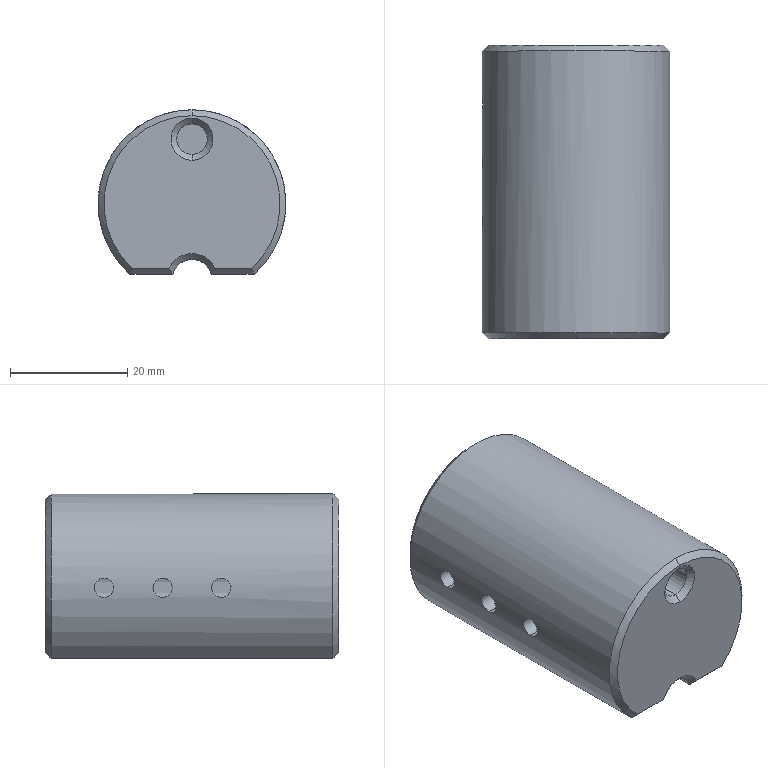Part | STEP file | 10000020504swp000-1 | 1 solid | 32 faces | box 32 x 50 x 28 mm | volume 27586 mm3 | cylinder 12 | cone 10 | plane 10 | commonest cylinder face diameters 3.3 x6 5.2 x2 15 x2 6.78 x1 32 x1
STEP:
#1=CARTESIAN_POINT('',(0.,49.,-9.49));
#2=VERTEX_POINT('',#1);
#3=CARTESIAN_POINT('',(3.274,49.,-12.));
#4=VERTEX_POINT('',#3);
#5=CARTESIAN_POINT('',(0.,49.,-12.88));
#6=DIRECTION('',(0.,1.,0.));
#7=DIRECTION('',(0.,0.,1.));
#8=AXIS2_PLACEMENT_3D('',#5,#6,#7);
#9=CIRCLE('',#8,3.39);
#10=EDGE_CURVE('',#2,#4,#9,.T.);
#11=ORIENTED_EDGE('',*,*,#10,.F.);
#12=CARTESIAN_POINT('',(0.,49.995,-8.495));
#13=VERTEX_POINT('',#12);
#14=CARTESIAN_POINT('',(0.,50.,-8.49));
#15=DIRECTION('',(0.,0.7071,0.7071));
#16=VECTOR('',#15,1000.);
#17=LINE('',#14,#16);
#18=EDGE_CURVE('',#2,#13,#17,.T.);
#19=ORIENTED_EDGE('',*,*,#18,.T.);
#20=CARTESIAN_POINT('',(0.2406,50.,-8.497));
#21=VERTEX_POINT('',#20);
#22=CARTESIAN_POINT('',(0.2406,50.,-8.497));
#23=CARTESIAN_POINT('',(0.1604,49.997,-8.496));
#24=CARTESIAN_POINT('',(0.08018,49.995,-8.495));
#25=CARTESIAN_POINT('',(0.,49.995,-8.495));
#26=B_SPLINE_CURVE_WITH_KNOTS('',3,(#22,#23,#24,#25),.UNSPECIFIED.,.F.,.F.,(4,4),(0.,0.0002406),.UNSPECIFIED.);
#27=EDGE_CURVE('',#21,#13,#26,.T.);
#28=ORIENTED_EDGE('',*,*,#27,.F.);
#29=CARTESIAN_POINT('',(3.967,50.,-11.));
#30=VERTEX_POINT('',#29);
#31=CARTESIAN_POINT('',(0.,50.,-12.88));
#32=DIRECTION('',(0.,-1.,0.));
#33=DIRECTION('',(0.,0.,1.));
#34=AXIS2_PLACEMENT_3D('',#31,#32,#33);
#35=CIRCLE('',#34,4.39);
#36=EDGE_CURVE('',#30,#21,#35,.T.);
#37=ORIENTED_EDGE('',*,*,#36,.F.);
#38=CARTESIAN_POINT('',(3.967,50.,-11.));
#39=CARTESIAN_POINT('',(3.753,49.661,-11.339));
#40=CARTESIAN_POINT('',(3.524,49.327,-11.673));
#41=CARTESIAN_POINT('',(3.274,49.,-12.));
#42=B_SPLINE_CURVE_WITH_KNOTS('',3,(#38,#39,#40,#41),.UNSPECIFIED.,.F.,.F.,(4,4),(0.,0.001575),.UNSPECIFIED.);
#43=EDGE_CURVE('',#30,#4,#42,.T.);
#44=ORIENTED_EDGE('',*,*,#43,.T.);
#45=EDGE_LOOP('',(#11,#19,#28,#37,#44));
#46=FACE_OUTER_BOUND('',#45,.T.);
#47=CARTESIAN_POINT('',(0.,50.,-12.88));
#48=DIRECTION('',(0.,1.,0.));
#49=DIRECTION('',(0.,0.,1.));
#50=AXIS2_PLACEMENT_3D('',#47,#48,#49);
#51=CONICAL_SURFACE('',#50,4.39,0.7854);
#52=ADVANCED_FACE('',(#46),#51,.F.);
#53=CARTESIAN_POINT('',(0.,49.,-7.5));
#54=VERTEX_POINT('',#53);
#55=CARTESIAN_POINT('',(0.,49.,7.5));
#56=VERTEX_POINT('',#55);
#57=CARTESIAN_POINT('',(0.,49.,0.));
#58=DIRECTION('',(0.,1.,0.));
#59=DIRECTION('',(0.,0.,1.));
#60=AXIS2_PLACEMENT_3D('',#57,#58,#59);
#61=CIRCLE('',#60,7.5);
#62=EDGE_CURVE('',#54,#56,#61,.T.);
#63=ORIENTED_EDGE('',*,*,#62,.F.);
#64=CARTESIAN_POINT('',(0.,49.,-7.5));
#65=DIRECTION('',(0.,0.7071,-0.7071));
#66=VECTOR('',#65,1000.);
#67=LINE('',#64,#66);
#68=EDGE_CURVE('',#54,#13,#67,.T.);
#69=ORIENTED_EDGE('',*,*,#68,.T.);
#70=CARTESIAN_POINT('',(-0.2406,50.,-8.497));
#71=VERTEX_POINT('',#70);
#72=CARTESIAN_POINT('',(0.,49.995,-8.495));
#73=CARTESIAN_POINT('',(-0.08018,49.995,-8.495));
#74=CARTESIAN_POINT('',(-0.1604,49.997,-8.496));
#75=CARTESIAN_POINT('',(-0.2406,50.,-8.497));
#76=B_SPLINE_CURVE_WITH_KNOTS('',3,(#72,#73,#74,#75),.UNSPECIFIED.,.F.,.F.,(4,4),(0.0002406,0.0004811),.UNSPECIFIED.);
#77=EDGE_CURVE('',#13,#71,#76,.T.);
#78=ORIENTED_EDGE('',*,*,#77,.T.);
#79=CARTESIAN_POINT('',(0.,50.,8.5));
#80=VERTEX_POINT('',#79);
#81=CARTESIAN_POINT('',(0.,50.,0.));
#82=DIRECTION('',(0.,-1.,0.));
#83=DIRECTION('',(0.,0.,1.));
#84=AXIS2_PLACEMENT_3D('',#81,#82,#83);
#85=CIRCLE('',#84,8.5);
#86=EDGE_CURVE('',#80,#71,#85,.T.);
#87=ORIENTED_EDGE('',*,*,#86,.F.);
#88=CARTESIAN_POINT('',(0.,49.,7.5));
#89=DIRECTION('',(0.,0.7071,0.7071));
#90=VECTOR('',#89,1000.);
#91=LINE('',#88,#90);
#92=EDGE_CURVE('',#56,#80,#91,.T.);
#93=ORIENTED_EDGE('',*,*,#92,.F.);
#94=EDGE_LOOP('',(#63,#69,#78,#87,#93));
#95=FACE_OUTER_BOUND('',#94,.T.);
#96=CARTESIAN_POINT('',(0.,49.,0.));
#97=DIRECTION('',(0.,1.,0.));
#98=DIRECTION('',(0.,0.,1.));
#99=AXIS2_PLACEMENT_3D('',#96,#97,#98);
#100=CONICAL_SURFACE('',#99,7.5,0.7854);
#101=ADVANCED_FACE('',(#95),#100,.F.);
#102=CARTESIAN_POINT('',(0.,1.,13.6));
#103=VERTEX_POINT('',#102);
#104=CARTESIAN_POINT('',(0.,1.,8.4));
#105=VERTEX_POINT('',#104);
#106=CARTESIAN_POINT('',(0.,1.,11.));
#107=DIRECTION('',(0.,-1.,0.));
#108=DIRECTION('',(0.,0.,1.));
#109=AXIS2_PLACEMENT_3D('',#106,#107,#108);
#110=CIRCLE('',#109,2.6);
#111=EDGE_CURVE('',#103,#105,#110,.T.);
#112=ORIENTED_EDGE('',*,*,#111,.F.);
#113=CARTESIAN_POINT('',(0.,0.,14.6));
#114=VERTEX_POINT('',#113);
#115=CARTESIAN_POINT('',(0.,1.,13.6));
#116=DIRECTION('',(0.,-0.7071,0.7071));
#117=VECTOR('',#116,1000.);
#118=LINE('',#115,#117);
#119=EDGE_CURVE('',#103,#114,#118,.T.);
#120=ORIENTED_EDGE('',*,*,#119,.T.);
#121=CARTESIAN_POINT('',(0.,0.,7.4));
#122=VERTEX_POINT('',#121);
#123=CARTESIAN_POINT('',(0.,0.,11.));
#124=DIRECTION('',(0.,1.,0.));
#125=DIRECTION('',(0.,0.,1.));
#126=AXIS2_PLACEMENT_3D('',#123,#124,#125);
#127=CIRCLE('',#126,3.6);
#128=EDGE_CURVE('',#122,#114,#127,.T.);
#129=ORIENTED_EDGE('',*,*,#128,.F.);
#130=CARTESIAN_POINT('',(0.,1.,8.4));
#131=DIRECTION('',(0.,-0.7071,-0.7071));
#132=VECTOR('',#131,1000.);
#133=LINE('',#130,#132);
#134=EDGE_CURVE('',#105,#122,#133,.T.);
#135=ORIENTED_EDGE('',*,*,#134,.F.);
#136=EDGE_LOOP('',(#112,#120,#129,#135));
#137=FACE_OUTER_BOUND('',#136,.T.);
#138=CARTESIAN_POINT('',(0.,1.,11.));
#139=DIRECTION('',(0.,-1.,0.));
#140=DIRECTION('',(0.,0.,-1.));
#141=AXIS2_PLACEMENT_3D('',#138,#139,#140);
#142=CONICAL_SURFACE('',#141,2.6,0.7854);
#143=ADVANCED_FACE('',(#137),#142,.F.);
#144=CARTESIAN_POINT('',(0.,0.,15.));
#145=VERTEX_POINT('',#144);
#146=CARTESIAN_POINT('',(-10.198,0.,-11.));
#147=VERTEX_POINT('',#146);
#148=CARTESIAN_POINT('',(0.,0.,0.));
#149=DIRECTION('',(0.,-1.,0.));
#150=DIRECTION('',(0.,0.,1.));
#151=AXIS2_PLACEMENT_3D('',#148,#149,#150);
#152=CIRCLE('',#151,15.);
#153=EDGE_CURVE('',#145,#147,#152,.T.);
#154=ORIENTED_EDGE('',*,*,#153,.F.);
#155=CARTESIAN_POINT('',(0.,1.,16.));
#156=VERTEX_POINT('',#155);
#157=CARTESIAN_POINT('',(0.,1.,16.));
#158=DIRECTION('',(0.,0.7071,0.7071));
#159=VECTOR('',#158,1000.);
#160=LINE('',#157,#159);
#161=EDGE_CURVE('',#145,#156,#160,.T.);
#162=ORIENTED_EDGE('',*,*,#161,.T.);
#163=CARTESIAN_POINT('',(-10.583,1.,-12.));
#164=VERTEX_POINT('',#163);
#165=CARTESIAN_POINT('',(0.,1.,0.));
#166=DIRECTION('',(0.,1.,0.));
#167=DIRECTION('',(0.,0.,1.));
#168=AXIS2_PLACEMENT_3D('',#165,#166,#167);
#169=CIRCLE('',#168,16.);
#170=EDGE_CURVE('',#164,#156,#169,.T.);
#171=ORIENTED_EDGE('',*,*,#170,.F.);
#172=CARTESIAN_POINT('',(-10.583,1.,-12.));
#173=CARTESIAN_POINT('',(-10.457,0.6663,-11.666));
#174=CARTESIAN_POINT('',(-10.329,0.3329,-11.333));
#175=CARTESIAN_POINT('',(-10.198,0.,-11.));
#176=B_SPLINE_CURVE_WITH_KNOTS('',3,(#172,#173,#174,#175),.UNSPECIFIED.,.F.,.F.,(4,4),(0.,0.001466),.UNSPECIFIED.);
#177=EDGE_CURVE('',#164,#147,#176,.T.);
#178=ORIENTED_EDGE('',*,*,#177,.T.);
#179=EDGE_LOOP('',(#154,#162,#171,#178));
#180=FACE_OUTER_BOUND('',#179,.T.);
#181=CARTESIAN_POINT('',(0.,1.,0.));
#182=DIRECTION('',(0.,1.,0.));
#183=DIRECTION('',(0.,0.,1.));
#184=AXIS2_PLACEMENT_3D('',#181,#182,#183);
#185=CONICAL_SURFACE('',#184,16.,0.7854);
#186=ADVANCED_FACE('',(#180),#185,.T.);
#187=CARTESIAN_POINT('',(-15.915,40.,1.65));
#188=VERTEX_POINT('',#187);
#189=CARTESIAN_POINT('',(-15.915,40.,-1.65));
#190=VERTEX_POINT('',#189);
#191=CARTESIAN_POINT('',(-15.915,40.,1.65));
#192=CARTESIAN_POINT('',(-15.915,39.785,1.65));
#193=CARTESIAN_POINT('',(-15.919,39.567,1.607));
#194=CARTESIAN_POINT('',(-15.935,39.17,1.442));
#195=CARTESIAN_POINT('',(-15.946,38.986,1.32));
#196=CARTESIAN_POINT('',(-15.963,38.758,1.092));
#197=CARTESIAN_POINT('',(-15.969,38.688,1.007));
#198=CARTESIAN_POINT('',(-15.979,38.568,0.8275));
#199=CARTESIAN_POINT('',(-15.984,38.518,0.7329));
#200=CARTESIAN_POINT('',(-15.991,38.435,0.5332));
#201=CARTESIAN_POINT('',(-15.995,38.403,0.4284));
#202=CARTESIAN_POINT('',(-15.999,38.361,0.2175));
#203=CARTESIAN_POINT('',(-16.,38.35,0.1103));
#204=CARTESIAN_POINT('',(-16.,38.35,-0.1078));
#205=CARTESIAN_POINT('',(-15.999,38.361,-0.2151));
#206=CARTESIAN_POINT('',(-15.995,38.402,-0.4261));
#207=CARTESIAN_POINT('',(-15.992,38.434,-0.5309));
#208=CARTESIAN_POINT('',(-15.984,38.517,-0.7308));
#209=CARTESIAN_POINT('',(-15.979,38.567,-0.8256));
#210=CARTESIAN_POINT('',(-15.969,38.687,-1.005));
#211=CARTESIAN_POINT('',(-15.963,38.756,-1.09));
#212=CARTESIAN_POINT('',(-15.946,38.984,-1.318));
#213=CARTESIAN_POINT('',(-15.935,39.168,-1.441));
#214=CARTESIAN_POINT('',(-15.919,39.565,-1.606));
#215=CARTESIAN_POINT('',(-15.915,39.782,-1.65));
#216=CARTESIAN_POINT('',(-15.915,40.,-1.65));
#217=B_SPLINE_CURVE_WITH_KNOTS('',3,(#191,#192,#193,#194,#195,#196,#197,#198,#199,#200,#201,#202,#203,#204,#205,#206,#207,#208,#209,#210,#211,#212,#213,#214,#215,#216),.UNSPECIFIED.,.F.,.F.,(4,2,2,2,2,2,2,2,2,2,2,2,4),(0.005162,0.005807,0.006452,0.006775,0.007097,0.00742,0.007743,0.008065,0.008388,0.00871,0.009033,0.009678,0.01032),.UNSPECIFIED.);
#218=EDGE_CURVE('',#188,#190,#217,.T.);
#219=ORIENTED_EDGE('',*,*,#218,.F.);
#220=CARTESIAN_POINT('',(-7.316,40.,1.65));
#221=VERTEX_POINT('',#220);
#222=CARTESIAN_POINT('',(0.,40.,1.65));
#223=DIRECTION('',(1.,0.,0.));
#224=VECTOR('',#223,1000.);
#225=LINE('',#222,#224);
#226=EDGE_CURVE('',#188,#221,#225,.T.);
#227=ORIENTED_EDGE('',*,*,#226,.T.);
#228=CARTESIAN_POINT('',(-7.316,40.,-1.65));
#229=VERTEX_POINT('',#228);
#230=CARTESIAN_POINT('',(-7.316,40.,-1.65));
#231=CARTESIAN_POINT('',(-7.316,39.891,-1.65));
#232=CARTESIAN_POINT('',(-7.319,39.783,-1.639));
#233=CARTESIAN_POINT('',(-7.328,39.572,-1.597));
#234=CARTESIAN_POINT('',(-7.335,39.467,-1.565));
#235=CARTESIAN_POINT('',(-7.352,39.267,-1.482));
#236=CARTESIAN_POINT('',(-7.362,39.172,-1.432));
#237=CARTESIAN_POINT('',(-7.385,38.993,-1.312));
#238=CARTESIAN_POINT('',(-7.397,38.909,-1.242));
#239=CARTESIAN_POINT('',(-7.433,38.681,-1.015));
#240=CARTESIAN_POINT('',(-7.456,38.559,-0.8311));
#241=CARTESIAN_POINT('',(-7.49,38.394,-0.4343));
#242=CARTESIAN_POINT('',(-7.5,38.35,-0.2166));
#243=CARTESIAN_POINT('',(-7.5,38.35,0.1073));
#244=CARTESIAN_POINT('',(-7.498,38.361,0.2171));
#245=CARTESIAN_POINT('',(-7.488,38.403,0.429));
#246=CARTESIAN_POINT('',(-7.482,38.434,0.532));
#247=CARTESIAN_POINT('',(-7.456,38.559,0.8323));
#248=CARTESIAN_POINT('',(-7.433,38.68,1.014));
#249=CARTESIAN_POINT('',(-7.397,38.91,1.244));
#250=CARTESIAN_POINT('',(-7.385,38.993,1.312));
#251=CARTESIAN_POINT('',(-7.362,39.171,1.431));
#252=CARTESIAN_POINT('',(-7.352,39.268,1.483));
#253=CARTESIAN_POINT('',(-7.335,39.467,1.565));
#254=CARTESIAN_POINT('',(-7.328,39.57,1.597));
#255=CARTESIAN_POINT('',(-7.319,39.783,1.639));
#256=CARTESIAN_POINT('',(-7.316,39.892,1.65));
#257=CARTESIAN_POINT('',(-7.316,40.,1.65));
#258=B_SPLINE_CURVE_WITH_KNOTS('',3,(#230,#231,#232,#233,#234,#235,#236,#237,#238,#239,#240,#241,#242,#243,#244,#245,#246,#247,#248,#249,#250,#251,#252,#253,#254,#255,#256,#257),.UNSPECIFIED.,.F.,.F.,(4,2,2,2,2,2,2,2,2,2,2,2,2,4),(0.,0.0003234,0.0006468,0.0009702,0.001294,0.00194,0.002587,0.002911,0.003234,0.003881,0.004204,0.004528,0.004851,0.005174),.UNSPECIFIED.);
#259=EDGE_CURVE('',#229,#221,#258,.T.);
#260=ORIENTED_EDGE('',*,*,#259,.F.);
#261=CARTESIAN_POINT('',(0.,40.,-1.65));
#262=DIRECTION('',(1.,0.,0.));
#263=VECTOR('',#262,1000.);
#264=LINE('',#261,#263);
#265=EDGE_CURVE('',#190,#229,#264,.T.);
#266=ORIENTED_EDGE('',*,*,#265,.F.);
#267=EDGE_LOOP('',(#219,#227,#260,#266));
#268=FACE_OUTER_BOUND('',#267,.T.);
#269=CARTESIAN_POINT('',(0.,40.,0.));
#270=DIRECTION('',(1.,0.,0.));
#271=DIRECTION('',(0.,0.,-1.));
#272=AXIS2_PLACEMENT_3D('',#269,#270,#271);
#273=CYLINDRICAL_SURFACE('',#272,1.65);
#274=ADVANCED_FACE('',(#268),#273,.F.);
#275=CARTESIAN_POINT('',(-15.915,30.,1.65));
#276=VERTEX_POINT('',#275);
#277=CARTESIAN_POINT('',(-15.915,30.,-1.65));
#278=VERTEX_POINT('',#277);
#279=CARTESIAN_POINT('',(-15.915,30.,1.65));
#280=CARTESIAN_POINT('',(-15.915,29.785,1.65));
#281=CARTESIAN_POINT('',(-15.919,29.567,1.607));
#282=CARTESIAN_POINT('',(-15.935,29.17,1.442));
#283=CARTESIAN_POINT('',(-15.946,28.986,1.32));
#284=CARTESIAN_POINT('',(-15.963,28.758,1.092));
#285=CARTESIAN_POINT('',(-15.969,28.688,1.007));
#286=CARTESIAN_POINT('',(-15.979,28.568,0.8275));
#287=CARTESIAN_POINT('',(-15.984,28.518,0.7329));
#288=CARTESIAN_POINT('',(-15.991,28.435,0.5332));
#289=CARTESIAN_POINT('',(-15.995,28.403,0.4284));
#290=CARTESIAN_POINT('',(-15.999,28.361,0.2175));
#291=CARTESIAN_POINT('',(-16.,28.35,0.1103));
#292=CARTESIAN_POINT('',(-16.,28.35,-0.1078));
#293=CARTESIAN_POINT('',(-15.999,28.361,-0.2151));
#294=CARTESIAN_POINT('',(-15.995,28.402,-0.4261));
#295=CARTESIAN_POINT('',(-15.992,28.434,-0.5309));
#296=CARTESIAN_POINT('',(-15.984,28.517,-0.7308));
#297=CARTESIAN_POINT('',(-15.979,28.567,-0.8256));
#298=CARTESIAN_POINT('',(-15.969,28.687,-1.005));
#299=CARTESIAN_POINT('',(-15.963,28.756,-1.09));
#300=CARTESIAN_POINT('',(-15.946,28.984,-1.318));
#301=CARTESIAN_POINT('',(-15.935,29.168,-1.441));
#302=CARTESIAN_POINT('',(-15.919,29.565,-1.606));
#303=CARTESIAN_POINT('',(-15.915,29.782,-1.65));
#304=CARTESIAN_POINT('',(-15.915,30.,-1.65));
#305=B_SPLINE_CURVE_WITH_KNOTS('',3,(#279,#280,#281,#282,#283,#284,#285,#286,#287,#288,#289,#290,#291,#292,#293,#294,#295,#296,#297,#298,#299,#300,#301,#302,#303,#304),.UNSPECIFIED.,.F.,.F.,(4,2,2,2,2,2,2,2,2,2,2,2,4),(0.005162,0.005807,0.006452,0.006775,0.007097,0.00742,0.007743,0.008065,0.008388,0.00871,0.009033,0.009678,0.01032),.UNSPECIFIED.);
#306=EDGE_CURVE('',#276,#278,#305,.T.);
#307=ORIENTED_EDGE('',*,*,#306,.F.);
#308=CARTESIAN_POINT('',(-7.316,30.,1.65));
#309=VERTEX_POINT('',#308);
#310=CARTESIAN_POINT('',(0.,30.,1.65));
#311=DIRECTION('',(1.,0.,0.));
#312=VECTOR('',#311,1000.);
#313=LINE('',#310,#312);
#314=EDGE_CURVE('',#276,#309,#313,.T.);
#315=ORIENTED_EDGE('',*,*,#314,.T.);
#316=CARTESIAN_POINT('',(-7.316,30.,-1.65));
#317=VERTEX_POINT('',#316);
#318=CARTESIAN_POINT('',(-7.316,30.,-1.65));
#319=CARTESIAN_POINT('',(-7.316,29.891,-1.65));
#320=CARTESIAN_POINT('',(-7.319,29.783,-1.639));
#321=CARTESIAN_POINT('',(-7.328,29.572,-1.597));
#322=CARTESIAN_POINT('',(-7.335,29.467,-1.565));
#323=CARTESIAN_POINT('',(-7.352,29.267,-1.482));
#324=CARTESIAN_POINT('',(-7.362,29.172,-1.432));
#325=CARTESIAN_POINT('',(-7.385,28.993,-1.312));
#326=CARTESIAN_POINT('',(-7.397,28.909,-1.242));
#327=CARTESIAN_POINT('',(-7.433,28.681,-1.015));
#328=CARTESIAN_POINT('',(-7.456,28.559,-0.8311));
#329=CARTESIAN_POINT('',(-7.49,28.394,-0.4343));
#330=CARTESIAN_POINT('',(-7.5,28.35,-0.2166));
#331=CARTESIAN_POINT('',(-7.5,28.35,0.1073));
#332=CARTESIAN_POINT('',(-7.498,28.361,0.2171));
#333=CARTESIAN_POINT('',(-7.488,28.403,0.429));
#334=CARTESIAN_POINT('',(-7.482,28.434,0.532));
#335=CARTESIAN_POINT('',(-7.456,28.559,0.8323));
#336=CARTESIAN_POINT('',(-7.433,28.68,1.014));
#337=CARTESIAN_POINT('',(-7.397,28.91,1.244));
#338=CARTESIAN_POINT('',(-7.385,28.993,1.312));
#339=CARTESIAN_POINT('',(-7.362,29.171,1.431));
#340=CARTESIAN_POINT('',(-7.352,29.268,1.483));
#341=CARTESIAN_POINT('',(-7.335,29.467,1.565));
#342=CARTESIAN_POINT('',(-7.328,29.57,1.597));
#343=CARTESIAN_POINT('',(-7.319,29.783,1.639));
#344=CARTESIAN_POINT('',(-7.316,29.892,1.65));
#345=CARTESIAN_POINT('',(-7.316,30.,1.65));
#346=B_SPLINE_CURVE_WITH_KNOTS('',3,(#318,#319,#320,#321,#322,#323,#324,#325,#326,#327,#328,#329,#330,#331,#332,#333,#334,#335,#336,#337,#338,#339,#340,#341,#342,#343,#344,#345),.UNSPECIFIED.,.F.,.F.,(4,2,2,2,2,2,2,2,2,2,2,2,2,4),(0.,0.0003234,0.0006468,0.0009702,0.001294,0.00194,0.002587,0.002911,0.003234,0.003881,0.004204,0.004528,0.004851,0.005174),.UNSPECIFIED.);
#347=EDGE_CURVE('',#317,#309,#346,.T.);
#348=ORIENTED_EDGE('',*,*,#347,.F.);
#349=CARTESIAN_POINT('',(0.,30.,-1.65));
#350=DIRECTION('',(1.,0.,0.));
#351=VECTOR('',#350,1000.);
#352=LINE('',#349,#351);
#353=EDGE_CURVE('',#278,#317,#352,.T.);
#354=ORIENTED_EDGE('',*,*,#353,.F.);
#355=EDGE_LOOP('',(#307,#315,#348,#354));
#356=FACE_OUTER_BOUND('',#355,.T.);
#357=CARTESIAN_POINT('',(0.,30.,0.));
#358=DIRECTION('',(1.,0.,0.));
#359=DIRECTION('',(0.,0.,-1.));
#360=AXIS2_PLACEMENT_3D('',#357,#358,#359);
#361=CYLINDRICAL_SURFACE('',#360,1.65);
#362=ADVANCED_FACE('',(#356),#361,.F.);
#363=CARTESIAN_POINT('',(-15.915,20.,1.65));
#364=VERTEX_POINT('',#363);
#365=CARTESIAN_POINT('',(-15.915,20.,-1.65));
#366=VERTEX_POINT('',#365);
#367=CARTESIAN_POINT('',(-15.915,20.,1.65));
#368=CARTESIAN_POINT('',(-15.915,19.785,1.65));
#369=CARTESIAN_POINT('',(-15.919,19.567,1.607));
#370=CARTESIAN_POINT('',(-15.935,19.17,1.442));
#371=CARTESIAN_POINT('',(-15.946,18.986,1.32));
#372=CARTESIAN_POINT('',(-15.963,18.758,1.092));
#373=CARTESIAN_POINT('',(-15.969,18.688,1.007));
#374=CARTESIAN_POINT('',(-15.979,18.568,0.8275));
#375=CARTESIAN_POINT('',(-15.984,18.518,0.7329));
#376=CARTESIAN_POINT('',(-15.991,18.435,0.5332));
#377=CARTESIAN_POINT('',(-15.995,18.403,0.4284));
#378=CARTESIAN_POINT('',(-15.999,18.361,0.2175));
#379=CARTESIAN_POINT('',(-16.,18.35,0.1103));
#380=CARTESIAN_POINT('',(-16.,18.35,-0.1078));
#381=CARTESIAN_POINT('',(-15.999,18.361,-0.2151));
#382=CARTESIAN_POINT('',(-15.995,18.402,-0.4261));
#383=CARTESIAN_POINT('',(-15.992,18.434,-0.5309));
#384=CARTESIAN_POINT('',(-15.984,18.517,-0.7308));
#385=CARTESIAN_POINT('',(-15.979,18.567,-0.8256));
#386=CARTESIAN_POINT('',(-15.969,18.687,-1.005));
#387=CARTESIAN_POINT('',(-15.963,18.756,-1.09));
#388=CARTESIAN_POINT('',(-15.946,18.984,-1.318));
#389=CARTESIAN_POINT('',(-15.935,19.168,-1.441));
#390=CARTESIAN_POINT('',(-15.919,19.565,-1.606));
#391=CARTESIAN_POINT('',(-15.915,19.782,-1.65));
#392=CARTESIAN_POINT('',(-15.915,20.,-1.65));
#393=B_SPLINE_CURVE_WITH_KNOTS('',3,(#367,#368,#369,#370,#371,#372,#373,#374,#375,#376,#377,#378,#379,#380,#381,#382,#383,#384,#385,#386,#387,#388,#389,#390,#391,#392),.UNSPECIFIED.,.F.,.F.,(4,2,2,2,2,2,2,2,2,2,2,2,4),(0.005162,0.005807,0.006452,0.006775,0.007097,0.00742,0.007743,0.008065,0.008388,0.00871,0.009033,0.009678,0.01032),.UNSPECIFIED.);
#394=EDGE_CURVE('',#364,#366,#393,.T.);
#395=ORIENTED_EDGE('',*,*,#394,.F.);
#396=CARTESIAN_POINT('',(-7.316,20.,1.65));
#397=VERTEX_POINT('',#396);
#398=CARTESIAN_POINT('',(0.,20.,1.65));
#399=DIRECTION('',(1.,0.,0.));
#400=VECTOR('',#399,1000.);
#401=LINE('',#398,#400);
#402=EDGE_CURVE('',#364,#397,#401,.T.);
#403=ORIENTED_EDGE('',*,*,#402,.T.);
#404=CARTESIAN_POINT('',(-7.316,20.,-1.65));
#405=VERTEX_POINT('',#404);
#406=CARTESIAN_POINT('',(-7.316,20.,-1.65));
#407=CARTESIAN_POINT('',(-7.316,19.891,-1.65));
#408=CARTESIAN_POINT('',(-7.319,19.783,-1.639));
#409=CARTESIAN_POINT('',(-7.328,19.572,-1.597));
#410=CARTESIAN_POINT('',(-7.335,19.467,-1.565));
#411=CARTESIAN_POINT('',(-7.352,19.267,-1.482));
#412=CARTESIAN_POINT('',(-7.362,19.172,-1.432));
#413=CARTESIAN_POINT('',(-7.385,18.993,-1.312));
#414=CARTESIAN_POINT('',(-7.397,18.909,-1.242));
#415=CARTESIAN_POINT('',(-7.433,18.681,-1.015));
#416=CARTESIAN_POINT('',(-7.456,18.559,-0.8311));
#417=CARTESIAN_POINT('',(-7.49,18.394,-0.4343));
#418=CARTESIAN_POINT('',(-7.5,18.35,-0.2166));
#419=CARTESIAN_POINT('',(-7.5,18.35,0.1073));
#420=CARTESIAN_POINT('',(-7.498,18.361,0.2171));
#421=CARTESIAN_POINT('',(-7.488,18.403,0.429));
#422=CARTESIAN_POINT('',(-7.482,18.434,0.532));
#423=CARTESIAN_POINT('',(-7.456,18.559,0.8323));
#424=CARTESIAN_POINT('',(-7.433,18.68,1.014));
#425=CARTESIAN_POINT('',(-7.397,18.91,1.244));
#426=CARTESIAN_POINT('',(-7.385,18.993,1.312));
#427=CARTESIAN_POINT('',(-7.362,19.171,1.431));
#428=CARTESIAN_POINT('',(-7.352,19.268,1.483));
#429=CARTESIAN_POINT('',(-7.335,19.467,1.565));
#430=CARTESIAN_POINT('',(-7.328,19.57,1.597));
#431=CARTESIAN_POINT('',(-7.319,19.783,1.639));
#432=CARTESIAN_POINT('',(-7.316,19.892,1.65));
#433=CARTESIAN_POINT('',(-7.316,20.,1.65));
#434=B_SPLINE_CURVE_WITH_KNOTS('',3,(#406,#407,#408,#409,#410,#411,#412,#413,#414,#415,#416,#417,#418,#419,#420,#421,#422,#423,#424,#425,#426,#427,#428,#429,#430,#431,#432,#433),.UNSPECIFIED.,.F.,.F.,(4,2,2,2,2,2,2,2,2,2,2,2,2,4),(0.,0.0003234,0.0006468,0.0009702,0.001294,0.00194,0.002587,0.002911,0.003234,0.003881,0.004204,0.004528,0.004851,0.005174),.UNSPECIFIED.);
#435=EDGE_CURVE('',#405,#397,#434,.T.);
#436=ORIENTED_EDGE('',*,*,#435,.F.);
#437=CARTESIAN_POINT('',(0.,20.,-1.65));
#438=DIRECTION('',(1.,0.,0.));
#439=VECTOR('',#438,1000.);
#440=LINE('',#437,#439);
#441=EDGE_CURVE('',#366,#405,#440,.T.);
#442=ORIENTED_EDGE('',*,*,#441,.F.);
#443=EDGE_LOOP('',(#395,#403,#436,#442));
#444=FACE_OUTER_BOUND('',#443,.T.);
#445=CARTESIAN_POINT('',(0.,20.,0.));
#446=DIRECTION('',(1.,0.,0.));
#447=DIRECTION('',(0.,0.,-1.));
#448=AXIS2_PLACEMENT_3D('',#445,#446,#447);
#449=CYLINDRICAL_SURFACE('',#448,1.65);
#450=ADVANCED_FACE('',(#444),#449,.F.);
#451=ORIENTED_EDGE('',*,*,#259,.T.);
#452=CARTESIAN_POINT('',(-7.316,40.,1.65));
#453=CARTESIAN_POINT('',(-7.316,40.216,1.65));
#454=CARTESIAN_POINT('',(-7.326,40.433,1.607));
#455=CARTESIAN_POINT('',(-7.352,40.731,1.483));
#456=CARTESIAN_POINT('',(-7.362,40.828,1.431));
#457=CARTESIAN_POINT('',(-7.385,41.007,1.311));
#458=CARTESIAN_POINT('',(-7.397,41.09,1.243));
#459=CARTESIAN_POINT('',(-7.421,41.242,1.091));
#460=CARTESIAN_POINT('',(-7.433,41.312,1.007));
#461=CARTESIAN_POINT('',(-7.455,41.431,0.8283));
#462=CARTESIAN_POINT('',(-7.465,41.482,0.7337));
#463=CARTESIAN_POINT('',(-7.49,41.607,0.4332));
#464=CARTESIAN_POINT('',(-7.5,41.65,0.2185));
#465=CARTESIAN_POINT('',(-7.5,41.65,-0.1082));
#466=CARTESIAN_POINT('',(-7.498,41.639,-0.2155));
#467=CARTESIAN_POINT('',(-7.489,41.597,-0.4271));
#468=CARTESIAN_POINT('',(-7.482,41.565,-0.5324));
#469=CARTESIAN_POINT('',(-7.456,41.442,-0.8312));
#470=CARTESIAN_POINT('',(-7.433,41.319,-1.014));
#471=CARTESIAN_POINT('',(-7.385,41.016,-1.318));
#472=CARTESIAN_POINT('',(-7.361,40.833,-1.441));
#473=CARTESIAN_POINT('',(-7.335,40.535,-1.565));
#474=CARTESIAN_POINT('',(-7.328,40.43,-1.597));
#475=CARTESIAN_POINT('',(-7.319,40.217,-1.639));
#476=CARTESIAN_POINT('',(-7.316,40.109,-1.65));
#477=CARTESIAN_POINT('',(-7.316,40.,-1.65));
#478=B_SPLINE_CURVE_WITH_KNOTS('',3,(#452,#453,#454,#455,#456,#457,#458,#459,#460,#461,#462,#463,#464,#465,#466,#467,#468,#469,#470,#471,#472,#473,#474,#475,#476,#477),.UNSPECIFIED.,.F.,.F.,(4,2,2,2,2,2,2,2,2,2,2,2,4),(0.005174,0.005821,0.006144,0.006468,0.006791,0.007114,0.007761,0.008084,0.008408,0.009054,0.009701,0.01002,0.01035),.UNSPECIFIED.);
#479=EDGE_CURVE('',#221,#229,#478,.T.);
#480=ORIENTED_EDGE('',*,*,#479,.T.);
#481=EDGE_LOOP('',(#451,#480));
#482=FACE_BOUND('',#481,.T.);
#483=ORIENTED_EDGE('',*,*,#347,.T.);
#484=CARTESIAN_POINT('',(-7.316,30.,1.65));
#485=CARTESIAN_POINT('',(-7.316,30.216,1.65));
#486=CARTESIAN_POINT('',(-7.326,30.433,1.607));
#487=CARTESIAN_POINT('',(-7.352,30.731,1.483));
#488=CARTESIAN_POINT('',(-7.362,30.828,1.431));
#489=CARTESIAN_POINT('',(-7.385,31.007,1.311));
#490=CARTESIAN_POINT('',(-7.397,31.09,1.243));
#491=CARTESIAN_POINT('',(-7.421,31.242,1.091));
#492=CARTESIAN_POINT('',(-7.433,31.312,1.007));
#493=CARTESIAN_POINT('',(-7.455,31.431,0.8283));
#494=CARTESIAN_POINT('',(-7.465,31.482,0.7337));
#495=CARTESIAN_POINT('',(-7.49,31.607,0.4332));
#496=CARTESIAN_POINT('',(-7.5,31.65,0.2185));
#497=CARTESIAN_POINT('',(-7.5,31.65,-0.1082));
#498=CARTESIAN_POINT('',(-7.498,31.639,-0.2155));
#499=CARTESIAN_POINT('',(-7.489,31.597,-0.4271));
#500=CARTESIAN_POINT('',(-7.482,31.565,-0.5324));
#501=CARTESIAN_POINT('',(-7.456,31.442,-0.8312));
#502=CARTESIAN_POINT('',(-7.433,31.319,-1.014));
#503=CARTESIAN_POINT('',(-7.385,31.016,-1.318));
#504=CARTESIAN_POINT('',(-7.361,30.833,-1.441));
#505=CARTESIAN_POINT('',(-7.335,30.535,-1.565));
#506=CARTESIAN_POINT('',(-7.328,30.43,-1.597));
#507=CARTESIAN_POINT('',(-7.319,30.217,-1.639));
#508=CARTESIAN_POINT('',(-7.316,30.109,-1.65));
#509=CARTESIAN_POINT('',(-7.316,30.,-1.65));
#510=B_SPLINE_CURVE_WITH_KNOTS('',3,(#484,#485,#486,#487,#488,#489,#490,#491,#492,#493,#494,#495,#496,#497,#498,#499,#500,#501,#502,#503,#504,#505,#506,#507,#508,#509),.UNSPECIFIED.,.F.,.F.,(4,2,2,2,2,2,2,2,2,2,2,2,4),(0.005174,0.005821,0.006144,0.006468,0.006791,0.007114,0.007761,0.008084,0.008408,0.009054,0.009701,0.01002,0.01035),.UNSPECIFIED.);
#511=EDGE_CURVE('',#309,#317,#510,.T.);
#512=ORIENTED_EDGE('',*,*,#511,.T.);
#513=EDGE_LOOP('',(#483,#512));
#514=FACE_BOUND('',#513,.T.);
#515=ORIENTED_EDGE('',*,*,#435,.T.);
#516=CARTESIAN_POINT('',(-7.316,20.,1.65));
#517=CARTESIAN_POINT('',(-7.316,20.216,1.65));
#518=CARTESIAN_POINT('',(-7.326,20.433,1.607));
#519=CARTESIAN_POINT('',(-7.352,20.731,1.483));
#520=CARTESIAN_POINT('',(-7.362,20.828,1.431));
#521=CARTESIAN_POINT('',(-7.385,21.007,1.311));
#522=CARTESIAN_POINT('',(-7.397,21.09,1.243));
#523=CARTESIAN_POINT('',(-7.421,21.242,1.091));
#524=CARTESIAN_POINT('',(-7.433,21.312,1.007));
#525=CARTESIAN_POINT('',(-7.455,21.431,0.8283));
#526=CARTESIAN_POINT('',(-7.465,21.482,0.7337));
#527=CARTESIAN_POINT('',(-7.49,21.607,0.4332));
#528=CARTESIAN_POINT('',(-7.5,21.65,0.2185));
#529=CARTESIAN_POINT('',(-7.5,21.65,-0.1082));
#530=CARTESIAN_POINT('',(-7.498,21.639,-0.2155));
#531=CARTESIAN_POINT('',(-7.489,21.597,-0.4271));
#532=CARTESIAN_POINT('',(-7.482,21.565,-0.5324));
#533=CARTESIAN_POINT('',(-7.456,21.442,-0.8312));
#534=CARTESIAN_POINT('',(-7.433,21.319,-1.014));
#535=CARTESIAN_POINT('',(-7.385,21.016,-1.318));
#536=CARTESIAN_POINT('',(-7.361,20.833,-1.441));
#537=CARTESIAN_POINT('',(-7.335,20.535,-1.565));
#538=CARTESIAN_POINT('',(-7.328,20.43,-1.597));
#539=CARTESIAN_POINT('',(-7.319,20.217,-1.639));
#540=CARTESIAN_POINT('',(-7.316,20.109,-1.65));
#541=CARTESIAN_POINT('',(-7.316,20.,-1.65));
#542=B_SPLINE_CURVE_WITH_KNOTS('',3,(#516,#517,#518,#519,#520,#521,#522,#523,#524,#525,#526,#527,#528,#529,#530,#531,#532,#533,#534,#535,#536,#537,#538,#539,#540,#541),.UNSPECIFIED.,.F.,.F.,(4,2,2,2,2,2,2,2,2,2,2,2,4),(0.005174,0.005821,0.006144,0.006468,0.006791,0.007114,0.007761,0.008084,0.008408,0.009054,0.009701,0.01002,0.01035),.UNSPECIFIED.);
#543=EDGE_CURVE('',#397,#405,#542,.T.);
#544=ORIENTED_EDGE('',*,*,#543,.T.);
#545=EDGE_LOOP('',(#515,#544));
#546=FACE_BOUND('',#545,.T.);
#547=CARTESIAN_POINT('',(0.,4.,-7.5));
#548=VERTEX_POINT('',#547);
#549=CARTESIAN_POINT('',(0.,4.,7.5));
#550=VERTEX_POINT('',#549);
#551=CARTESIAN_POINT('',(0.,4.,0.));
#552=DIRECTION('',(0.,1.,0.));
#553=DIRECTION('',(0.,0.,1.));
#554=AXIS2_PLACEMENT_3D('',#551,#552,#553);
#555=CIRCLE('',#554,7.5);
#556=EDGE_CURVE('',#548,#550,#555,.T.);
#557=ORIENTED_EDGE('',*,*,#556,.F.);
#558=CARTESIAN_POINT('',(0.,50.,-7.5));
#559=DIRECTION('',(0.,1.,0.));
#560=VECTOR('',#559,1000.);
#561=LINE('',#558,#560);
#562=EDGE_CURVE('',#548,#54,#561,.T.);
#563=ORIENTED_EDGE('',*,*,#562,.T.);
#564=ORIENTED_EDGE('',*,*,#62,.T.);
#565=CARTESIAN_POINT('',(0.,50.,7.5));
#566=DIRECTION('',(0.,1.,0.));
#567=VECTOR('',#566,1000.);
#568=LINE('',#565,#567);
#569=EDGE_CURVE('',#550,#56,#568,.T.);
#570=ORIENTED_EDGE('',*,*,#569,.F.);
#571=EDGE_LOOP('',(#557,#563,#564,#570));
#572=FACE_OUTER_BOUND('',#571,.T.);
#573=CARTESIAN_POINT('',(0.,50.,0.));
#574=DIRECTION('',(0.,1.,0.));
#575=DIRECTION('',(0.,0.,1.));
#576=AXIS2_PLACEMENT_3D('',#573,#574,#575);
#577=CYLINDRICAL_SURFACE('',#576,7.5);
#578=ADVANCED_FACE('',(#482,#514,#546,#572),#577,.F.);
#579=CARTESIAN_POINT('',(0.,30.,13.6));
#580=VERTEX_POINT('',#579);
#581=CARTESIAN_POINT('',(0.,30.,8.4));
#582=VERTEX_POINT('',#581);
#583=CARTESIAN_POINT('',(0.,30.,11.));
#584=DIRECTION('',(0.,-1.,0.));
#585=DIRECTION('',(0.,0.,-1.));
#586=AXIS2_PLACEMENT_3D('',#583,#584,#585);
#587=CIRCLE('',#586,2.6);
#588=EDGE_CURVE('',#580,#582,#587,.T.);
#589=ORIENTED_EDGE('',*,*,#588,.F.);
#590=CARTESIAN_POINT('',(0.,0.,13.6));
#591=DIRECTION('',(0.,-1.,0.));
#592=VECTOR('',#591,1000.);
#593=LINE('',#590,#592);
#594=EDGE_CURVE('',#580,#103,#593,.T.);
#595=ORIENTED_EDGE('',*,*,#594,.T.);
#596=ORIENTED_EDGE('',*,*,#111,.T.);
#597=CARTESIAN_POINT('',(0.,0.,8.4));
#598=DIRECTION('',(0.,-1.,0.));
#599=VECTOR('',#598,1000.);
#600=LINE('',#597,#599);
#601=EDGE_CURVE('',#582,#105,#600,.T.);
#602=ORIENTED_EDGE('',*,*,#601,.F.);
#603=EDGE_LOOP('',(#589,#595,#596,#602));
#604=FACE_OUTER_BOUND('',#603,.T.);
#605=CARTESIAN_POINT('',(0.,0.,11.));
#606=DIRECTION('',(0.,-1.,0.));
#607=DIRECTION('',(0.,0.,-1.));
#608=AXIS2_PLACEMENT_3D('',#605,#606,#607);
#609=CYLINDRICAL_SURFACE('',#608,2.6);
#610=ADVANCED_FACE('',(#604),#609,.F.);
#611=CARTESIAN_POINT('',(10.583,49.,-12.));
#612=VERTEX_POINT('',#611);
#613=CARTESIAN_POINT('',(10.583,1.,-12.));
#614=VERTEX_POINT('',#613);
#615=CARTESIAN_POINT('',(10.583,50.,-12.));
#616=DIRECTION('',(0.,-1.,0.));
#617=VECTOR('',#616,1000.);
#618=LINE('',#615,#617);
#619=EDGE_CURVE('',#612,#614,#618,.T.);
#620=ORIENTED_EDGE('',*,*,#619,.T.);
#621=CARTESIAN_POINT('',(3.274,1.,-12.));
#622=VERTEX_POINT('',#621);
#623=CARTESIAN_POINT('',(3.274,1.,-12.));
#624=DIRECTION('',(-1.,0.,0.));
#625=VECTOR('',#624,1000.);
#626=LINE('',#623,#625);
#627=EDGE_CURVE('',#614,#622,#626,.T.);
#628=ORIENTED_EDGE('',*,*,#627,.T.);
#629=CARTESIAN_POINT('',(3.274,50.,-12.));
#630=DIRECTION('',(0.,-1.,0.));
#631=VECTOR('',#630,1000.);
#632=LINE('',#629,#631);
#633=EDGE_CURVE('',#4,#622,#632,.T.);
#634=ORIENTED_EDGE('',*,*,#633,.F.);
#635=CARTESIAN_POINT('',(-10.583,49.,-12.));
#636=DIRECTION('',(1.,0.,0.));
#637=VECTOR('',#636,1000.);
#638=LINE('',#635,#637);
#639=EDGE_CURVE('',#4,#612,#638,.T.);
#640=ORIENTED_EDGE('',*,*,#639,.T.);
#641=EDGE_LOOP('',(#620,#628,#634,#640));
#642=FACE_OUTER_BOUND('',#641,.T.);
#643=CARTESIAN_POINT('',(-10.583,50.,-12.));
#644=DIRECTION('',(0.,0.,-1.));
#645=DIRECTION('',(-1.,0.,0.));
#646=AXIS2_PLACEMENT_3D('',#643,#644,#645);
#647=PLANE('',#646);
#648=ADVANCED_FACE('',(#642),#647,.T.);
#649=CARTESIAN_POINT('',(-15.915,40.,-1.65));
#650=CARTESIAN_POINT('',(-15.915,40.109,-1.65));
#651=CARTESIAN_POINT('',(-15.916,40.216,-1.639));
#652=CARTESIAN_POINT('',(-15.92,40.427,-1.597));
#653=CARTESIAN_POINT('',(-15.923,40.532,-1.566));
#654=CARTESIAN_POINT('',(-15.931,40.732,-1.483));
#655=CARTESIAN_POINT('',(-15.936,40.827,-1.432));
#656=CARTESIAN_POINT('',(-15.946,41.006,-1.312));
#657=CARTESIAN_POINT('',(-15.952,41.091,-1.243));
#658=CARTESIAN_POINT('',(-15.969,41.319,-1.014));
#659=CARTESIAN_POINT('',(-15.98,41.442,-0.8303));
#660=CARTESIAN_POINT('',(-15.995,41.607,-0.4333));
#661=CARTESIAN_POINT('',(-16.,41.65,-0.216));
#662=CARTESIAN_POINT('',(-16.,41.65,0.1071));
#663=CARTESIAN_POINT('',(-15.999,41.639,0.2165));
#664=CARTESIAN_POINT('',(-15.995,41.597,0.4282));
#665=CARTESIAN_POINT('',(-15.991,41.566,0.5311));
#666=CARTESIAN_POINT('',(-15.984,41.483,0.7309));
#667=CARTESIAN_POINT('',(-15.979,41.432,0.8275));
#668=CARTESIAN_POINT('',(-15.969,41.312,1.006));
#669=CARTESIAN_POINT('',(-15.963,41.244,1.09));
#670=CARTESIAN_POINT('',(-15.952,41.09,1.244));
#671=CARTESIAN_POINT('',(-15.946,41.007,1.312));
#672=CARTESIAN_POINT('',(-15.936,40.828,1.431));
#673=CARTESIAN_POINT('',(-15.931,40.731,1.483));
#674=CARTESIAN_POINT('',(-15.923,40.532,1.566));
#675=CARTESIAN_POINT('',(-15.92,40.429,1.597));
#676=CARTESIAN_POINT('',(-15.916,40.217,1.639));
#677=CARTESIAN_POINT('',(-15.915,40.108,1.65));
#678=CARTESIAN_POINT('',(-15.915,40.,1.65));
#679=B_SPLINE_CURVE_WITH_KNOTS('',3,(#649,#650,#651,#652,#653,#654,#655,#656,#657,#658,#659,#660,#661,#662,#663,#664,#665,#666,#667,#668,#669,#670,#671,#672,#673,#674,#675,#676,#677,#678),.UNSPECIFIED.,.F.,.F.,(4,2,2,2,2,2,2,2,2,2,2,2,2,2,4),(0.,0.0003226,0.0006453,0.0009679,0.001291,0.001936,0.002581,0.002904,0.003226,0.003549,0.003872,0.004194,0.004517,0.004839,0.005162),.UNSPECIFIED.);
#680=EDGE_CURVE('',#190,#188,#679,.T.);
#681=ORIENTED_EDGE('',*,*,#680,.T.);
#682=ORIENTED_EDGE('',*,*,#218,.T.);
#683=EDGE_LOOP('',(#681,#682));
#684=FACE_BOUND('',#683,.T.);
#685=CARTESIAN_POINT('',(-15.915,30.,-1.65));
#686=CARTESIAN_POINT('',(-15.915,30.109,-1.65));
#687=CARTESIAN_POINT('',(-15.916,30.216,-1.639));
#688=CARTESIAN_POINT('',(-15.92,30.427,-1.597));
#689=CARTESIAN_POINT('',(-15.923,30.532,-1.566));
#690=CARTESIAN_POINT('',(-15.931,30.732,-1.483));
#691=CARTESIAN_POINT('',(-15.936,30.827,-1.432));
#692=CARTESIAN_POINT('',(-15.946,31.006,-1.312));
#693=CARTESIAN_POINT('',(-15.952,31.091,-1.243));
#694=CARTESIAN_POINT('',(-15.969,31.319,-1.014));
#695=CARTESIAN_POINT('',(-15.98,31.442,-0.8303));
#696=CARTESIAN_POINT('',(-15.995,31.607,-0.4333));
#697=CARTESIAN_POINT('',(-16.,31.65,-0.216));
#698=CARTESIAN_POINT('',(-16.,31.65,0.1071));
#699=CARTESIAN_POINT('',(-15.999,31.639,0.2165));
#700=CARTESIAN_POINT('',(-15.995,31.597,0.4282));
#701=CARTESIAN_POINT('',(-15.991,31.566,0.5311));
#702=CARTESIAN_POINT('',(-15.984,31.483,0.7309));
#703=CARTESIAN_POINT('',(-15.979,31.432,0.8275));
#704=CARTESIAN_POINT('',(-15.969,31.312,1.006));
#705=CARTESIAN_POINT('',(-15.963,31.244,1.09));
#706=CARTESIAN_POINT('',(-15.952,31.09,1.244));
#707=CARTESIAN_POINT('',(-15.946,31.007,1.312));
#708=CARTESIAN_POINT('',(-15.936,30.828,1.431));
#709=CARTESIAN_POINT('',(-15.931,30.731,1.483));
#710=CARTESIAN_POINT('',(-15.923,30.532,1.566));
#711=CARTESIAN_POINT('',(-15.92,30.429,1.597));
#712=CARTESIAN_POINT('',(-15.916,30.217,1.639));
#713=CARTESIAN_POINT('',(-15.915,30.108,1.65));
#714=CARTESIAN_POINT('',(-15.915,30.,1.65));
#715=B_SPLINE_CURVE_WITH_KNOTS('',3,(#685,#686,#687,#688,#689,#690,#691,#692,#693,#694,#695,#696,#697,#698,#699,#700,#701,#702,#703,#704,#705,#706,#707,#708,#709,#710,#711,#712,#713,#714),.UNSPECIFIED.,.F.,.F.,(4,2,2,2,2,2,2,2,2,2,2,2,2,2,4),(0.,0.0003226,0.0006453,0.0009679,0.001291,0.001936,0.002581,0.002904,0.003226,0.003549,0.003872,0.004194,0.004517,0.004839,0.005162),.UNSPECIFIED.);
#716=EDGE_CURVE('',#278,#276,#715,.T.);
#717=ORIENTED_EDGE('',*,*,#716,.T.);
#718=ORIENTED_EDGE('',*,*,#306,.T.);
#719=EDGE_LOOP('',(#717,#718));
#720=FACE_BOUND('',#719,.T.);
#721=CARTESIAN_POINT('',(-15.915,20.,-1.65));
#722=CARTESIAN_POINT('',(-15.915,20.109,-1.65));
#723=CARTESIAN_POINT('',(-15.916,20.216,-1.639));
#724=CARTESIAN_POINT('',(-15.92,20.427,-1.597));
#725=CARTESIAN_POINT('',(-15.923,20.532,-1.566));
#726=CARTESIAN_POINT('',(-15.931,20.732,-1.483));
#727=CARTESIAN_POINT('',(-15.936,20.827,-1.432));
#728=CARTESIAN_POINT('',(-15.946,21.006,-1.312));
#729=CARTESIAN_POINT('',(-15.952,21.091,-1.243));
#730=CARTESIAN_POINT('',(-15.969,21.319,-1.014));
#731=CARTESIAN_POINT('',(-15.98,21.442,-0.8303));
#732=CARTESIAN_POINT('',(-15.995,21.607,-0.4333));
#733=CARTESIAN_POINT('',(-16.,21.65,-0.216));
#734=CARTESIAN_POINT('',(-16.,21.65,0.1071));
#735=CARTESIAN_POINT('',(-15.999,21.639,0.2165));
#736=CARTESIAN_POINT('',(-15.995,21.597,0.4282));
#737=CARTESIAN_POINT('',(-15.991,21.566,0.5311));
#738=CARTESIAN_POINT('',(-15.984,21.483,0.7309));
#739=CARTESIAN_POINT('',(-15.979,21.432,0.8275));
#740=CARTESIAN_POINT('',(-15.969,21.312,1.006));
#741=CARTESIAN_POINT('',(-15.963,21.244,1.09));
#742=CARTESIAN_POINT('',(-15.952,21.09,1.244));
#743=CARTESIAN_POINT('',(-15.946,21.007,1.312));
#744=CARTESIAN_POINT('',(-15.936,20.828,1.431));
#745=CARTESIAN_POINT('',(-15.931,20.731,1.483));
#746=CARTESIAN_POINT('',(-15.923,20.532,1.566));
#747=CARTESIAN_POINT('',(-15.92,20.429,1.597));
#748=CARTESIAN_POINT('',(-15.916,20.217,1.639));
#749=CARTESIAN_POINT('',(-15.915,20.108,1.65));
#750=CARTESIAN_POINT('',(-15.915,20.,1.65));
#751=B_SPLINE_CURVE_WITH_KNOTS('',3,(#721,#722,#723,#724,#725,#726,#727,#728,#729,#730,#731,#732,#733,#734,#735,#736,#737,#738,#739,#740,#741,#742,#743,#744,#745,#746,#747,#748,#749,#750),.UNSPECIFIED.,.F.,.F.,(4,2,2,2,2,2,2,2,2,2,2,2,2,2,4),(0.,0.0003226,0.0006453,0.0009679,0.001291,0.001936,0.002581,0.002904,0.003226,0.003549,0.003872,0.004194,0.004517,0.004839,0.005162),.UNSPECIFIED.);
#752=EDGE_CURVE('',#366,#364,#751,.T.);
#753=ORIENTED_EDGE('',*,*,#752,.T.);
#754=ORIENTED_EDGE('',*,*,#394,.T.);
#755=EDGE_LOOP('',(#753,#754));
#756=FACE_BOUND('',#755,.T.);
#757=CARTESIAN_POINT('',(-10.583,49.,-12.));
#758=VERTEX_POINT('',#757);
#759=CARTESIAN_POINT('',(-10.583,50.,-12.));
#760=DIRECTION('',(0.,-1.,0.));
#761=VECTOR('',#760,1000.);
#762=LINE('',#759,#761);
#763=EDGE_CURVE('',#758,#164,#762,.T.);
#764=ORIENTED_EDGE('',*,*,#763,.T.);
#765=ORIENTED_EDGE('',*,*,#170,.T.);
#766=CARTESIAN_POINT('',(0.,1.,0.));
#767=DIRECTION('',(0.,1.,0.));
#768=DIRECTION('',(0.,0.,1.));
#769=AXIS2_PLACEMENT_3D('',#766,#767,#768);
#770=CIRCLE('',#769,16.);
#771=EDGE_CURVE('',#156,#614,#770,.T.);
#772=ORIENTED_EDGE('',*,*,#771,.T.);
#773=ORIENTED_EDGE('',*,*,#619,.F.);
#774=CARTESIAN_POINT('',(0.,49.,0.));
#775=DIRECTION('',(0.,-1.,0.));
#776=DIRECTION('',(0.,0.,1.));
#777=AXIS2_PLACEMENT_3D('',#774,#775,#776);
#778=CIRCLE('',#777,16.);
#779=EDGE_CURVE('',#612,#758,#778,.T.);
#780=ORIENTED_EDGE('',*,*,#779,.T.);
#781=EDGE_LOOP('',(#764,#765,#772,#773,#780));
#782=FACE_OUTER_BOUND('',#781,.T.);
#783=CARTESIAN_POINT('',(0.,50.,0.));
#784=DIRECTION('',(0.,-1.,0.));
#785=DIRECTION('',(0.,0.,-1.));
#786=AXIS2_PLACEMENT_3D('',#783,#784,#785);
#787=CYLINDRICAL_SURFACE('',#786,16.);
#788=ADVANCED_FACE('',(#684,#720,#756,#782),#787,.T.);
#789=CARTESIAN_POINT('',(-3.967,50.,-11.));
#790=VERTEX_POINT('',#789);
#791=CARTESIAN_POINT('',(0.,50.,-12.88));
#792=DIRECTION('',(0.,-1.,0.));
#793=DIRECTION('',(0.,0.,1.));
#794=AXIS2_PLACEMENT_3D('',#791,#792,#793);
#795=CIRCLE('',#794,4.39);
#796=EDGE_CURVE('',#71,#790,#795,.T.);
#797=ORIENTED_EDGE('',*,*,#796,.T.);
#798=CARTESIAN_POINT('',(-10.198,50.,-11.));
#799=VERTEX_POINT('',#798);
#800=CARTESIAN_POINT('',(0.,50.,-11.));
#801=DIRECTION('',(-1.,0.,0.));
#802=VECTOR('',#801,1000.);
#803=LINE('',#800,#802);
#804=EDGE_CURVE('',#790,#799,#803,.T.);
#805=ORIENTED_EDGE('',*,*,#804,.T.);
#806=CARTESIAN_POINT('',(10.198,50.,-11.));
#807=VERTEX_POINT('',#806);
#808=CARTESIAN_POINT('',(0.,50.,0.));
#809=DIRECTION('',(0.,1.,0.));
#810=DIRECTION('',(0.,0.,1.));
#811=AXIS2_PLACEMENT_3D('',#808,#809,#810);
#812=CIRCLE('',#811,15.);
#813=EDGE_CURVE('',#799,#807,#812,.T.);
#814=ORIENTED_EDGE('',*,*,#813,.T.);
#815=CARTESIAN_POINT('',(0.,50.,-11.));
#816=DIRECTION('',(-1.,0.,0.));
#817=VECTOR('',#816,1000.);
#818=LINE('',#815,#817);
#819=EDGE_CURVE('',#807,#30,#818,.T.);
#820=ORIENTED_EDGE('',*,*,#819,.T.);
#821=ORIENTED_EDGE('',*,*,#36,.T.);
#822=CARTESIAN_POINT('',(0.,50.,0.));
#823=DIRECTION('',(0.,-1.,0.));
#824=DIRECTION('',(0.,0.,1.));
#825=AXIS2_PLACEMENT_3D('',#822,#823,#824);
#826=CIRCLE('',#825,8.5);
#827=EDGE_CURVE('',#21,#80,#826,.T.);
#828=ORIENTED_EDGE('',*,*,#827,.T.);
#829=ORIENTED_EDGE('',*,*,#86,.T.);
#830=EDGE_LOOP('',(#797,#805,#814,#820,#821,#828,#829));
#831=FACE_OUTER_BOUND('',#830,.T.);
#832=CARTESIAN_POINT('',(0.,50.,0.));
#833=DIRECTION('',(0.,1.,0.));
#834=DIRECTION('',(0.,0.,1.));
#835=AXIS2_PLACEMENT_3D('',#832,#833,#834);
#836=PLANE('',#835);
#837=ADVANCED_FACE('',(#831),#836,.T.);
#838=ORIENTED_EDGE('',*,*,#128,.T.);
#839=CARTESIAN_POINT('',(0.,0.,11.));
#840=DIRECTION('',(0.,1.,0.));
#841=DIRECTION('',(0.,0.,1.));
#842=AXIS2_PLACEMENT_3D('',#839,#840,#841);
#843=CIRCLE('',#842,3.6);
#844=EDGE_CURVE('',#114,#122,#843,.T.);
#845=ORIENTED_EDGE('',*,*,#844,.T.);
#846=EDGE_LOOP('',(#838,#845));
#847=FACE_BOUND('',#846,.T.);
#848=CARTESIAN_POINT('',(10.198,0.,-11.));
#849=VERTEX_POINT('',#848);
#850=CARTESIAN_POINT('',(0.,0.,0.));
#851=DIRECTION('',(0.,-1.,0.));
#852=DIRECTION('',(0.,0.,1.));
#853=AXIS2_PLACEMENT_3D('',#850,#851,#852);
#854=CIRCLE('',#853,15.);
#855=EDGE_CURVE('',#849,#145,#854,.T.);
#856=ORIENTED_EDGE('',*,*,#855,.T.);
#857=ORIENTED_EDGE('',*,*,#153,.T.);
#858=CARTESIAN_POINT('',(-3.967,0.,-11.));
#859=VERTEX_POINT('',#858);
#860=CARTESIAN_POINT('',(-3.274,0.,-11.));
#861=DIRECTION('',(1.,0.,0.));
#862=VECTOR('',#861,1000.);
#863=LINE('',#860,#862);
#864=EDGE_CURVE('',#147,#859,#863,.T.);
#865=ORIENTED_EDGE('',*,*,#864,.T.);
#866=CARTESIAN_POINT('',(3.967,0.,-11.));
#867=VERTEX_POINT('',#866);
#868=CARTESIAN_POINT('',(0.,0.,-12.88));
#869=DIRECTION('',(0.,1.,0.));
#870=DIRECTION('',(0.,0.,1.));
#871=AXIS2_PLACEMENT_3D('',#868,#869,#870);
#872=CIRCLE('',#871,4.39);
#873=EDGE_CURVE('',#859,#867,#872,.T.);
#874=ORIENTED_EDGE('',*,*,#873,.T.);
#875=CARTESIAN_POINT('',(9.,0.,-11.));
#876=DIRECTION('',(1.,0.,0.));
#877=VECTOR('',#876,1000.);
#878=LINE('',#875,#877);
#879=EDGE_CURVE('',#867,#849,#878,.T.);
#880=ORIENTED_EDGE('',*,*,#879,.T.);
#881=EDGE_LOOP('',(#856,#857,#865,#874,#880));
#882=FACE_OUTER_BOUND('',#881,.T.);
#883=CARTESIAN_POINT('',(0.,0.,0.));
#884=DIRECTION('',(0.,1.,0.));
#885=DIRECTION('',(0.,0.,1.));
#886=AXIS2_PLACEMENT_3D('',#883,#884,#885);
#887=PLANE('',#886);
#888=ADVANCED_FACE('',(#847,#882),#887,.F.);
#889=CARTESIAN_POINT('',(-3.274,1.,-12.));
#890=VERTEX_POINT('',#889);
#891=CARTESIAN_POINT('',(-3.274,49.,-12.));
#892=VERTEX_POINT('',#891);
#893=CARTESIAN_POINT('',(-3.274,50.,-12.));
#894=DIRECTION('',(0.,1.,0.));
#895=VECTOR('',#894,1000.);
#896=LINE('',#893,#895);
#897=EDGE_CURVE('',#890,#892,#896,.T.);
#898=ORIENTED_EDGE('',*,*,#897,.F.);
#899=CARTESIAN_POINT('',(-9.,1.,-12.));
#900=DIRECTION('',(-1.,0.,0.));
#901=VECTOR('',#900,1000.);
#902=LINE('',#899,#901);
#903=EDGE_CURVE('',#890,#164,#902,.T.);
#904=ORIENTED_EDGE('',*,*,#903,.T.);
#905=ORIENTED_EDGE('',*,*,#763,.F.);
#906=CARTESIAN_POINT('',(-10.583,49.,-12.));
#907=DIRECTION('',(1.,0.,0.));
#908=VECTOR('',#907,1000.);
#909=LINE('',#906,#908);
#910=EDGE_CURVE('',#758,#892,#909,.T.);
#911=ORIENTED_EDGE('',*,*,#910,.T.);
#912=EDGE_LOOP('',(#898,#904,#905,#911));
#913=FACE_OUTER_BOUND('',#912,.T.);
#914=CARTESIAN_POINT('',(-10.583,50.,-12.));
#915=DIRECTION('',(0.,0.,-1.));
#916=DIRECTION('',(-1.,0.,0.));
#917=AXIS2_PLACEMENT_3D('',#914,#915,#916);
#918=PLANE('',#917);
#919=ADVANCED_FACE('',(#913),#918,.T.);
#920=ORIENTED_EDGE('',*,*,#633,.T.);
#921=CARTESIAN_POINT('',(0.,1.,-12.88));
#922=DIRECTION('',(0.,-1.,0.));
#923=DIRECTION('',(0.,0.,1.));
#924=AXIS2_PLACEMENT_3D('',#921,#922,#923);
#925=CIRCLE('',#924,3.39);
#926=EDGE_CURVE('',#622,#890,#925,.T.);
#927=ORIENTED_EDGE('',*,*,#926,.T.);
#928=ORIENTED_EDGE('',*,*,#897,.T.);
#929=CARTESIAN_POINT('',(0.,49.,-12.88));
#930=DIRECTION('',(0.,1.,0.));
#931=DIRECTION('',(0.,0.,1.));
#932=AXIS2_PLACEMENT_3D('',#929,#930,#931);
#933=CIRCLE('',#932,3.39);
#934=EDGE_CURVE('',#892,#2,#933,.T.);
#935=ORIENTED_EDGE('',*,*,#934,.T.);
#936=ORIENTED_EDGE('',*,*,#10,.T.);
#937=EDGE_LOOP('',(#920,#927,#928,#935,#936));
#938=FACE_OUTER_BOUND('',#937,.T.);
#939=CARTESIAN_POINT('',(0.,50.,-12.88));
#940=DIRECTION('',(0.,-1.,0.));
#941=DIRECTION('',(0.,0.,-1.));
#942=AXIS2_PLACEMENT_3D('',#939,#940,#941);
#943=CYLINDRICAL_SURFACE('',#942,3.39);
#944=ADVANCED_FACE('',(#938),#943,.F.);
#945=CARTESIAN_POINT('',(0.,30.,11.));
#946=DIRECTION('',(0.,-1.,0.));
#947=DIRECTION('',(0.,0.,-1.));
#948=AXIS2_PLACEMENT_3D('',#945,#946,#947);
#949=CIRCLE('',#948,2.6);
#950=EDGE_CURVE('',#582,#580,#949,.T.);
#951=ORIENTED_EDGE('',*,*,#950,.T.);
#952=ORIENTED_EDGE('',*,*,#588,.T.);
#953=EDGE_LOOP('',(#951,#952));
#954=FACE_OUTER_BOUND('',#953,.T.);
#955=CARTESIAN_POINT('',(0.,30.,11.));
#956=DIRECTION('',(0.,1.,0.));
#957=DIRECTION('',(0.,0.,1.));
#958=AXIS2_PLACEMENT_3D('',#955,#956,#957);
#959=PLANE('',#958);
#960=ADVANCED_FACE('',(#954),#959,.F.);
#961=ORIENTED_EDGE('',*,*,#594,.F.);
#962=ORIENTED_EDGE('',*,*,#950,.F.);
#963=ORIENTED_EDGE('',*,*,#601,.T.);
#964=CARTESIAN_POINT('',(0.,1.,11.));
#965=DIRECTION('',(0.,-1.,0.));
#966=DIRECTION('',(0.,0.,1.));
#967=AXIS2_PLACEMENT_3D('',#964,#965,#966);
#968=CIRCLE('',#967,2.6);
#969=EDGE_CURVE('',#105,#103,#968,.T.);
#970=ORIENTED_EDGE('',*,*,#969,.T.);
#971=EDGE_LOOP('',(#961,#962,#963,#970));
#972=FACE_OUTER_BOUND('',#971,.T.);
#973=CARTESIAN_POINT('',(0.,0.,11.));
#974=DIRECTION('',(0.,-1.,0.));
#975=DIRECTION('',(0.,0.,-1.));
#976=AXIS2_PLACEMENT_3D('',#973,#974,#975);
#977=CYLINDRICAL_SURFACE('',#976,2.6);
#978=ADVANCED_FACE('',(#972),#977,.F.);
#979=CARTESIAN_POINT('',(0.,4.,0.));
#980=DIRECTION('',(0.,1.,0.));
#981=DIRECTION('',(0.,0.,1.));
#982=AXIS2_PLACEMENT_3D('',#979,#980,#981);
#983=CIRCLE('',#982,7.5);
#984=EDGE_CURVE('',#550,#548,#983,.T.);
#985=ORIENTED_EDGE('',*,*,#984,.T.);
#986=ORIENTED_EDGE('',*,*,#556,.T.);
#987=EDGE_LOOP('',(#985,#986));
#988=FACE_OUTER_BOUND('',#987,.T.);
#989=CARTESIAN_POINT('',(0.,4.,0.));
#990=DIRECTION('',(0.,-1.,0.));
#991=DIRECTION('',(0.,0.,-1.));
#992=AXIS2_PLACEMENT_3D('',#989,#990,#991);
#993=PLANE('',#992);
#994=ADVANCED_FACE('',(#988),#993,.F.);
#995=ORIENTED_EDGE('',*,*,#562,.F.);
#996=ORIENTED_EDGE('',*,*,#984,.F.);
#997=ORIENTED_EDGE('',*,*,#569,.T.);
#998=CARTESIAN_POINT('',(0.,49.,0.));
#999=DIRECTION('',(0.,1.,0.));
#1000=DIRECTION('',(0.,0.,1.));
#1001=AXIS2_PLACEMENT_3D('',#998,#999,#1000);
#1002=CIRCLE('',#1001,7.5);
#1003=EDGE_CURVE('',#56,#54,#1002,.T.);
#1004=ORIENTED_EDGE('',*,*,#1003,.T.);
#1005=EDGE_LOOP('',(#995,#996,#997,#1004));
#1006=FACE_OUTER_BOUND('',#1005,.T.);
#1007=CARTESIAN_POINT('',(0.,50.,0.));
#1008=DIRECTION('',(0.,1.,0.));
#1009=DIRECTION('',(0.,0.,1.));
#1010=AXIS2_PLACEMENT_3D('',#1007,#1008,#1009);
#1011=CYLINDRICAL_SURFACE('',#1010,7.5);
#1012=ADVANCED_FACE('',(#1006),#1011,.F.);
#1013=ORIENTED_EDGE('',*,*,#402,.F.);
#1014=ORIENTED_EDGE('',*,*,#752,.F.);
#1015=ORIENTED_EDGE('',*,*,#441,.T.);
#1016=ORIENTED_EDGE('',*,*,#543,.F.);
#1017=EDGE_LOOP('',(#1013,#1014,#1015,#1016));
#1018=FACE_OUTER_BOUND('',#1017,.T.);
#1019=CARTESIAN_POINT('',(0.,20.,0.));
#1020=DIRECTION('',(1.,0.,0.));
#1021=DIRECTION('',(0.,0.,-1.));
#1022=AXIS2_PLACEMENT_3D('',#1019,#1020,#1021);
#1023=CYLINDRICAL_SURFACE('',#1022,1.65);
#1024=ADVANCED_FACE('',(#1018),#1023,.F.);
#1025=ORIENTED_EDGE('',*,*,#314,.F.);
#1026=ORIENTED_EDGE('',*,*,#716,.F.);
#1027=ORIENTED_EDGE('',*,*,#353,.T.);
#1028=ORIENTED_EDGE('',*,*,#511,.F.);
#1029=EDGE_LOOP('',(#1025,#1026,#1027,#1028));
#1030=FACE_OUTER_BOUND('',#1029,.T.);
#1031=CARTESIAN_POINT('',(0.,30.,0.));
#1032=DIRECTION('',(1.,0.,0.));
#1033=DIRECTION('',(0.,0.,-1.));
#1034=AXIS2_PLACEMENT_3D('',#1031,#1032,#1033);
#1035=CYLINDRICAL_SURFACE('',#1034,1.65);
#1036=ADVANCED_FACE('',(#1030),#1035,.F.);
#1037=ORIENTED_EDGE('',*,*,#226,.F.);
#1038=ORIENTED_EDGE('',*,*,#680,.F.);
#1039=ORIENTED_EDGE('',*,*,#265,.T.);
#1040=ORIENTED_EDGE('',*,*,#479,.F.);
#1041=EDGE_LOOP('',(#1037,#1038,#1039,#1040));
#1042=FACE_OUTER_BOUND('',#1041,.T.);
#1043=CARTESIAN_POINT('',(0.,40.,0.));
#1044=DIRECTION('',(1.,0.,0.));
#1045=DIRECTION('',(0.,0.,-1.));
#1046=AXIS2_PLACEMENT_3D('',#1043,#1044,#1045);
#1047=CYLINDRICAL_SURFACE('',#1046,1.65);
#1048=ADVANCED_FACE('',(#1042),#1047,.F.);
#1049=ORIENTED_EDGE('',*,*,#161,.F.);
#1050=ORIENTED_EDGE('',*,*,#855,.F.);
#1051=CARTESIAN_POINT('',(10.198,0.,-11.));
#1052=CARTESIAN_POINT('',(10.329,0.3329,-11.333));
#1053=CARTESIAN_POINT('',(10.457,0.6663,-11.666));
#1054=CARTESIAN_POINT('',(10.583,1.,-12.));
#1055=B_SPLINE_CURVE_WITH_KNOTS('',3,(#1051,#1052,#1053,#1054),.UNSPECIFIED.,.F.,.F.,(4,4),(0.,0.001466),.UNSPECIFIED.);
#1056=EDGE_CURVE('',#849,#614,#1055,.T.);
#1057=ORIENTED_EDGE('',*,*,#1056,.T.);
#1058=ORIENTED_EDGE('',*,*,#771,.F.);
#1059=EDGE_LOOP('',(#1049,#1050,#1057,#1058));
#1060=FACE_OUTER_BOUND('',#1059,.T.);
#1061=CARTESIAN_POINT('',(0.,1.,0.));
#1062=DIRECTION('',(0.,1.,0.));
#1063=DIRECTION('',(0.,0.,1.));
#1064=AXIS2_PLACEMENT_3D('',#1061,#1062,#1063);
#1065=CONICAL_SURFACE('',#1064,16.,0.7854);
#1066=ADVANCED_FACE('',(#1060),#1065,.T.);
#1067=ORIENTED_EDGE('',*,*,#119,.F.);
#1068=ORIENTED_EDGE('',*,*,#969,.F.);
#1069=ORIENTED_EDGE('',*,*,#134,.T.);
#1070=ORIENTED_EDGE('',*,*,#844,.F.);
#1071=EDGE_LOOP('',(#1067,#1068,#1069,#1070));
#1072=FACE_OUTER_BOUND('',#1071,.T.);
#1073=CARTESIAN_POINT('',(0.,1.,11.));
#1074=DIRECTION('',(0.,-1.,0.));
#1075=DIRECTION('',(0.,0.,-1.));
#1076=AXIS2_PLACEMENT_3D('',#1073,#1074,#1075);
#1077=CONICAL_SURFACE('',#1076,2.6,0.7854);
#1078=ADVANCED_FACE('',(#1072),#1077,.F.);
#1079=ORIENTED_EDGE('',*,*,#68,.F.);
#1080=ORIENTED_EDGE('',*,*,#1003,.F.);
#1081=ORIENTED_EDGE('',*,*,#92,.T.);
#1082=ORIENTED_EDGE('',*,*,#827,.F.);
#1083=ORIENTED_EDGE('',*,*,#27,.T.);
#1084=EDGE_LOOP('',(#1079,#1080,#1081,#1082,#1083));
#1085=FACE_OUTER_BOUND('',#1084,.T.);
#1086=CARTESIAN_POINT('',(0.,49.,0.));
#1087=DIRECTION('',(0.,1.,0.));
#1088=DIRECTION('',(0.,0.,1.));
#1089=AXIS2_PLACEMENT_3D('',#1086,#1087,#1088);
#1090=CONICAL_SURFACE('',#1089,7.5,0.7854);
#1091=ADVANCED_FACE('',(#1085),#1090,.F.);
#1092=ORIENTED_EDGE('',*,*,#813,.F.);
#1093=CARTESIAN_POINT('',(-10.198,50.,-11.));
#1094=CARTESIAN_POINT('',(-10.329,49.667,-11.333));
#1095=CARTESIAN_POINT('',(-10.457,49.334,-11.666));
#1096=CARTESIAN_POINT('',(-10.583,49.,-12.));
#1097=B_SPLINE_CURVE_WITH_KNOTS('',3,(#1093,#1094,#1095,#1096),.UNSPECIFIED.,.F.,.F.,(4,4),(0.,0.001466),.UNSPECIFIED.);
#1098=EDGE_CURVE('',#799,#758,#1097,.T.);
#1099=ORIENTED_EDGE('',*,*,#1098,.T.);
#1100=ORIENTED_EDGE('',*,*,#779,.F.);
#1101=CARTESIAN_POINT('',(10.583,49.,-12.));
#1102=CARTESIAN_POINT('',(10.457,49.334,-11.666));
#1103=CARTESIAN_POINT('',(10.329,49.667,-11.333));
#1104=CARTESIAN_POINT('',(10.198,50.,-11.));
#1105=B_SPLINE_CURVE_WITH_KNOTS('',3,(#1101,#1102,#1103,#1104),.UNSPECIFIED.,.F.,.F.,(4,4),(0.,0.001466),.UNSPECIFIED.);
#1106=EDGE_CURVE('',#612,#807,#1105,.T.);
#1107=ORIENTED_EDGE('',*,*,#1106,.T.);
#1108=EDGE_LOOP('',(#1092,#1099,#1100,#1107));
#1109=FACE_OUTER_BOUND('',#1108,.T.);
#1110=CARTESIAN_POINT('',(0.,50.,0.));
#1111=DIRECTION('',(0.,-1.,0.));
#1112=DIRECTION('',(0.,0.,-1.));
#1113=AXIS2_PLACEMENT_3D('',#1110,#1111,#1112);
#1114=CONICAL_SURFACE('',#1113,15.,0.7854);
#1115=ADVANCED_FACE('',(#1109),#1114,.T.);
#1116=ORIENTED_EDGE('',*,*,#1056,.F.);
#1117=ORIENTED_EDGE('',*,*,#879,.F.);
#1118=CARTESIAN_POINT('',(3.274,1.,-12.));
#1119=CARTESIAN_POINT('',(3.524,0.6734,-11.673));
#1120=CARTESIAN_POINT('',(3.753,0.3391,-11.339));
#1121=CARTESIAN_POINT('',(3.967,0.,-11.));
#1122=B_SPLINE_CURVE_WITH_KNOTS('',3,(#1118,#1119,#1120,#1121),.UNSPECIFIED.,.F.,.F.,(4,4),(0.,0.001575),.UNSPECIFIED.);
#1123=EDGE_CURVE('',#622,#867,#1122,.T.);
#1124=ORIENTED_EDGE('',*,*,#1123,.F.);
#1125=ORIENTED_EDGE('',*,*,#627,.F.);
#1126=EDGE_LOOP('',(#1116,#1117,#1124,#1125));
#1127=FACE_OUTER_BOUND('',#1126,.T.);
#1128=CARTESIAN_POINT('',(0.,0.,-11.));
#1129=DIRECTION('',(0.,-0.7071,-0.7071));
#1130=DIRECTION('',(-1.,0.,0.));
#1131=AXIS2_PLACEMENT_3D('',#1128,#1129,#1130);
#1132=PLANE('',#1131);
#1133=ADVANCED_FACE('',(#1127),#1132,.T.);
#1134=ORIENTED_EDGE('',*,*,#1123,.T.);
#1135=ORIENTED_EDGE('',*,*,#873,.F.);
#1136=CARTESIAN_POINT('',(-3.274,1.,-12.));
#1137=CARTESIAN_POINT('',(-3.524,0.6734,-11.673));
#1138=CARTESIAN_POINT('',(-3.753,0.3391,-11.339));
#1139=CARTESIAN_POINT('',(-3.967,0.,-11.));
#1140=B_SPLINE_CURVE_WITH_KNOTS('',3,(#1136,#1137,#1138,#1139),.UNSPECIFIED.,.F.,.F.,(4,4),(0.,0.001575),.UNSPECIFIED.);
#1141=EDGE_CURVE('',#890,#859,#1140,.T.);
#1142=ORIENTED_EDGE('',*,*,#1141,.F.);
#1143=ORIENTED_EDGE('',*,*,#926,.F.);
#1144=EDGE_LOOP('',(#1134,#1135,#1142,#1143));
#1145=FACE_OUTER_BOUND('',#1144,.T.);
#1146=CARTESIAN_POINT('',(0.,1.,-12.88));
#1147=DIRECTION('',(0.,-1.,0.));
#1148=DIRECTION('',(0.,0.,-1.));
#1149=AXIS2_PLACEMENT_3D('',#1146,#1147,#1148);
#1150=CONICAL_SURFACE('',#1149,3.39,0.7854);
#1151=ADVANCED_FACE('',(#1145),#1150,.F.);
#1152=ORIENTED_EDGE('',*,*,#177,.F.);
#1153=ORIENTED_EDGE('',*,*,#903,.F.);
#1154=ORIENTED_EDGE('',*,*,#1141,.T.);
#1155=ORIENTED_EDGE('',*,*,#864,.F.);
#1156=EDGE_LOOP('',(#1152,#1153,#1154,#1155));
#1157=FACE_OUTER_BOUND('',#1156,.T.);
#1158=CARTESIAN_POINT('',(0.,0.,-11.));
#1159=DIRECTION('',(0.,-0.7071,-0.7071));
#1160=DIRECTION('',(-1.,0.,0.));
#1161=AXIS2_PLACEMENT_3D('',#1158,#1159,#1160);
#1162=PLANE('',#1161);
#1163=ADVANCED_FACE('',(#1157),#1162,.T.);
#1164=ORIENTED_EDGE('',*,*,#1106,.F.);
#1165=ORIENTED_EDGE('',*,*,#639,.F.);
#1166=ORIENTED_EDGE('',*,*,#43,.F.);
#1167=ORIENTED_EDGE('',*,*,#819,.F.);
#1168=EDGE_LOOP('',(#1164,#1165,#1166,#1167));
#1169=FACE_OUTER_BOUND('',#1168,.T.);
#1170=CARTESIAN_POINT('',(-10.583,49.,-12.));
#1171=DIRECTION('',(0.,-0.7071,0.7071));
#1172=DIRECTION('',(1.,0.,0.));
#1173=AXIS2_PLACEMENT_3D('',#1170,#1171,#1172);
#1174=PLANE('',#1173);
#1175=ADVANCED_FACE('',(#1169),#1174,.F.);
#1176=ORIENTED_EDGE('',*,*,#18,.F.);
#1177=ORIENTED_EDGE('',*,*,#934,.F.);
#1178=CARTESIAN_POINT('',(-3.967,50.,-11.));
#1179=CARTESIAN_POINT('',(-3.753,49.661,-11.339));
#1180=CARTESIAN_POINT('',(-3.524,49.327,-11.673));
#1181=CARTESIAN_POINT('',(-3.274,49.,-12.));
#1182=B_SPLINE_CURVE_WITH_KNOTS('',3,(#1178,#1179,#1180,#1181),.UNSPECIFIED.,.F.,.F.,(4,4),(0.,0.001575),.UNSPECIFIED.);
#1183=EDGE_CURVE('',#790,#892,#1182,.T.);
#1184=ORIENTED_EDGE('',*,*,#1183,.F.);
#1185=ORIENTED_EDGE('',*,*,#796,.F.);
#1186=ORIENTED_EDGE('',*,*,#77,.F.);
#1187=EDGE_LOOP('',(#1176,#1177,#1184,#1185,#1186));
#1188=FACE_OUTER_BOUND('',#1187,.T.);
#1189=CARTESIAN_POINT('',(0.,50.,-12.88));
#1190=DIRECTION('',(0.,1.,0.));
#1191=DIRECTION('',(0.,0.,1.));
#1192=AXIS2_PLACEMENT_3D('',#1189,#1190,#1191);
#1193=CONICAL_SURFACE('',#1192,4.39,0.7854);
#1194=ADVANCED_FACE('',(#1188),#1193,.F.);
#1195=ORIENTED_EDGE('',*,*,#1098,.F.);
#1196=ORIENTED_EDGE('',*,*,#804,.F.);
#1197=ORIENTED_EDGE('',*,*,#1183,.T.);
#1198=ORIENTED_EDGE('',*,*,#910,.F.);
#1199=EDGE_LOOP('',(#1195,#1196,#1197,#1198));
#1200=FACE_OUTER_BOUND('',#1199,.T.);
#1201=CARTESIAN_POINT('',(-10.583,49.,-12.));
#1202=DIRECTION('',(0.,-0.7071,0.7071));
#1203=DIRECTION('',(1.,0.,0.));
#1204=AXIS2_PLACEMENT_3D('',#1201,#1202,#1203);
#1205=PLANE('',#1204);
#1206=ADVANCED_FACE('',(#1200),#1205,.F.);
#1207=CLOSED_SHELL('',(#52,#101,#143,#186,#274,#362,#450,#578,#610,#648,#788,#837,#888,#919,#944,#960,#978,#994,#1012,#1024,#1036,#1048,#1066,#1078,#1091,#1115,#1133,#1151,#1163,#1175,#1194,#1206));
#1208=MANIFOLD_SOLID_BREP('',#1207);
#1209=CARTESIAN_POINT('',(0.,0.,0.));
#1210=DIRECTION('',(0.,0.,1.));
#1211=DIRECTION('',(1.,0.,0.));
#1212=AXIS2_PLACEMENT_3D('',#1209,#1210,#1211);
#1213=(LENGTH_UNIT()NAMED_UNIT(*)SI_UNIT(.MILLI.,.METRE.));
#1214=UNCERTAINTY_MEASURE_WITH_UNIT(LENGTH_MEASURE(0.00001),#1213,'','');
#1215=(NAMED_UNIT(*)PLANE_ANGLE_UNIT()SI_UNIT($,.RADIAN.));
#1216=(NAMED_UNIT(*)SI_UNIT($,.STERADIAN.)SOLID_ANGLE_UNIT());
#1217=(GEOMETRIC_REPRESENTATION_CONTEXT(3)GLOBAL_UNCERTAINTY_ASSIGNED_CONTEXT((#1214))GLOBAL_UNIT_ASSIGNED_CONTEXT((#1213,#1215,#1216))REPRESENTATION_CONTEXT('',''));
#1218=ADVANCED_BREP_SHAPE_REPRESENTATION('',(#1208,#1212),#1217);